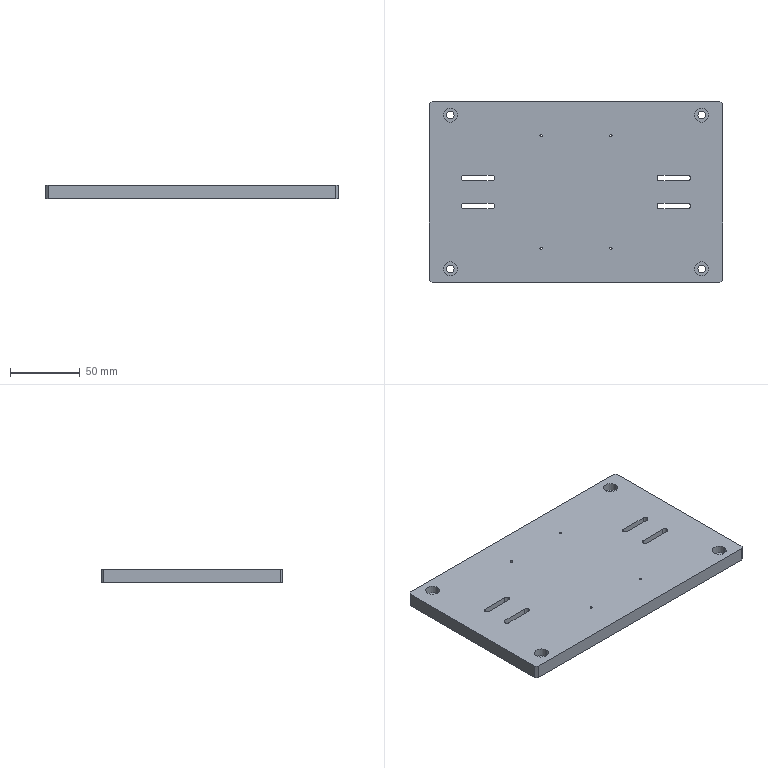Part | SolidWorks | features 3DProfileFeature 2, HoleWzd 2, Chamfer 1, Cut 1, Extrusion 1 | 1 solid | 58 faces | box 210 x 130 x 10 mm | volume 266938 mm3 | cylinder 36 | plane 22 | commonest cylinder face diameters 4 x12 1.6 x8 5.5 x8 10 x8